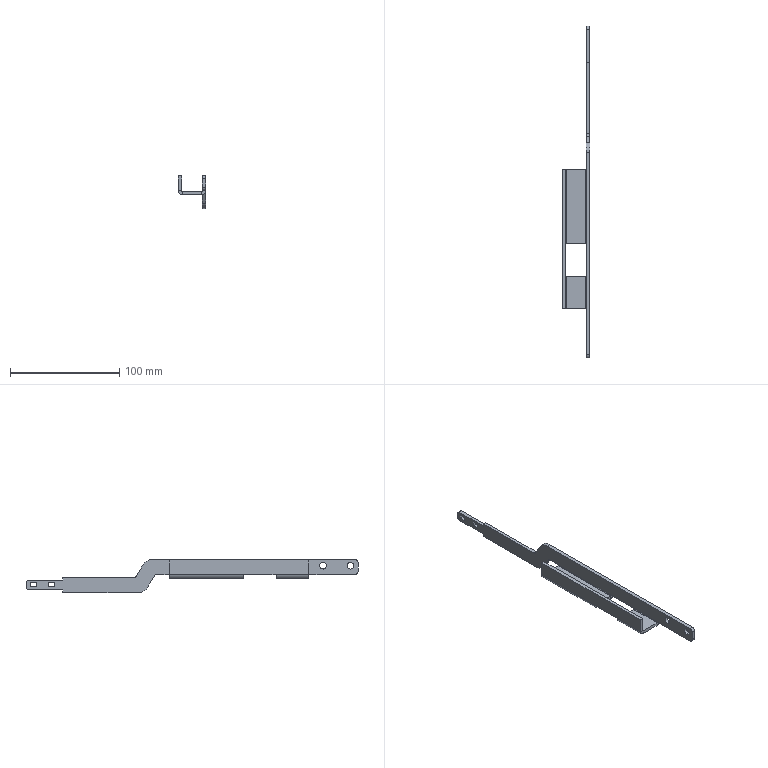Part | SolidWorks | features BaseBody 1 | 1 solid | 63 faces | box 25 x 304 x 30.5 mm | volume 24628 mm3 | plane 43 | cylinder 20 | commonest cylinder face diameters 6 x10 1 x4 7 x4 20 x2